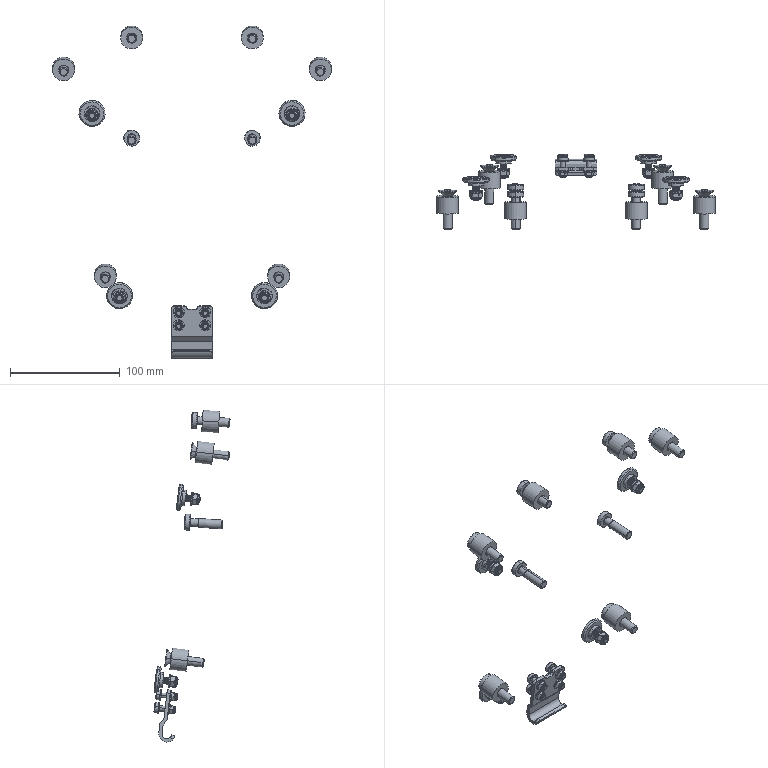Part | SolidWorks | 51 solids | 2079 faces | box 254 x 69.361 x 302.677 mm | volume 62240 mm3 | cylinder 701 | spline 468 | cone 392 | plane 270 | torus 240 | sphere 8 | commonest cylinder face diameters 6 x145 5 x71 1 x60 3.2 x39 1.01 x36 1.53 x32